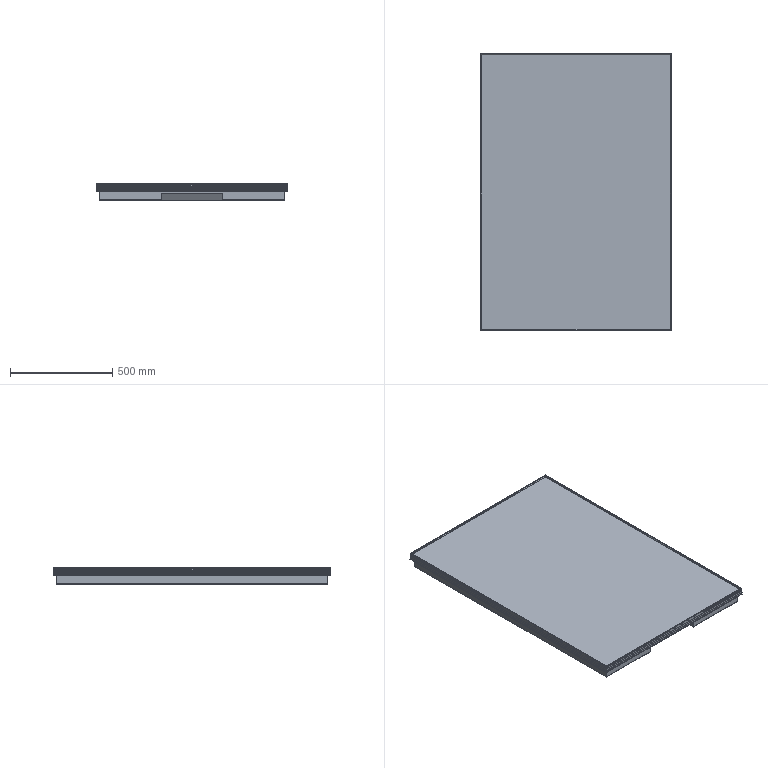Part | SolidWorks | 8 solids | 408 faces | box 940 x 1360 x 80 mm | volume 6967858 mm3 | plane 254 | cylinder 142 | spline 12 | commonest cylinder face diameters 7 x100 11 x16 1 x9 3 x9 5 x4 0.4 x2